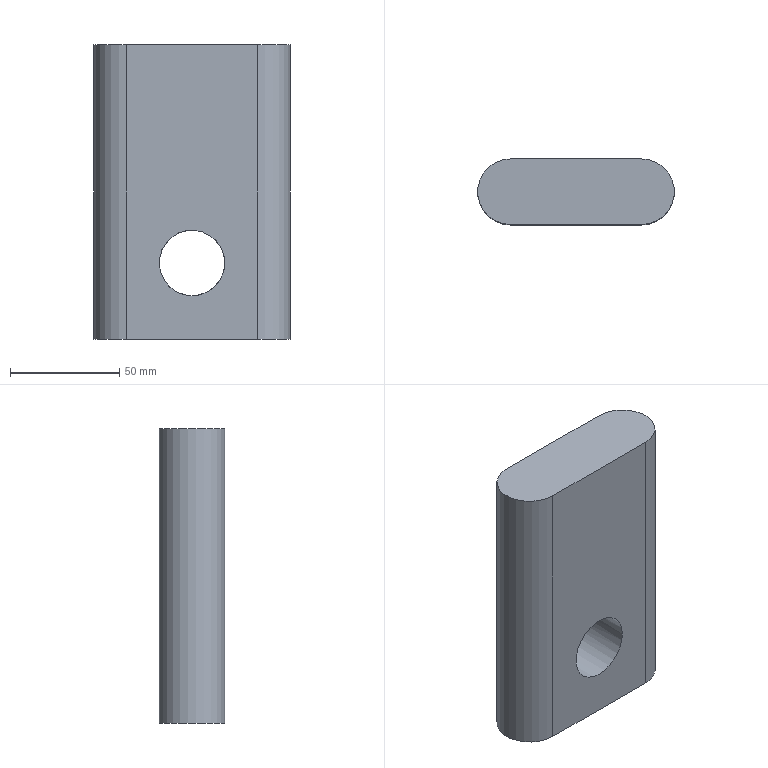Part | NX | features DATUM_CSYS 3, EXTRUDE 2, OFFSET_REGION 2, SKETCH 2, BLEND 1 | 1 solid | 7 faces | box 90 x 30 x 135 mm | volume 317220 mm3 | plane 4 | cylinder 3 | commonest cylinder face diameters 30 x3
STEP:
#1=CARTESIAN_POINT('',(15.,-15.,40.));
#2=VERTEX_POINT('',#1);
#3=CARTESIAN_POINT('',(0.,-15.,40.));
#4=DIRECTION('',(0.,-1.,0.));
#5=DIRECTION('',(1.,0.,0.));
#6=AXIS2_PLACEMENT_3D('',#3,#4,#5);
#7=CIRCLE('',#6,15.);
#8=EDGE_CURVE('',#2,#2,#7,.T.);
#9=ORIENTED_EDGE('',*,*,#8,.F.);
#10=EDGE_LOOP('',(#9));
#11=FACE_BOUND('',#10,.T.);
#12=CARTESIAN_POINT('',(-30.,-15.,5.));
#13=VERTEX_POINT('',#12);
#14=CARTESIAN_POINT('',(30.,-15.,5.));
#15=VERTEX_POINT('',#14);
#16=CARTESIAN_POINT('',(-45.,-15.,5.));
#17=DIRECTION('',(1.,0.,0.));
#18=VECTOR('',#17,1000.);
#19=LINE('',#16,#18);
#20=EDGE_CURVE('',#13,#15,#19,.T.);
#21=ORIENTED_EDGE('',*,*,#20,.T.);
#22=CARTESIAN_POINT('',(30.,-15.,140.));
#23=VERTEX_POINT('',#22);
#24=CARTESIAN_POINT('',(30.,-15.,100.));
#25=DIRECTION('',(0.,0.,-1.));
#26=VECTOR('',#25,1000.);
#27=LINE('',#24,#26);
#28=EDGE_CURVE('',#15,#23,#27,.F.);
#29=ORIENTED_EDGE('',*,*,#28,.T.);
#30=CARTESIAN_POINT('',(-30.,-15.,140.));
#31=VERTEX_POINT('',#30);
#32=CARTESIAN_POINT('',(-45.,-15.,140.));
#33=DIRECTION('',(1.,0.,0.));
#34=VECTOR('',#33,1000.);
#35=LINE('',#32,#34);
#36=EDGE_CURVE('',#31,#23,#35,.T.);
#37=ORIENTED_EDGE('',*,*,#36,.F.);
#38=CARTESIAN_POINT('',(-30.,-15.,100.));
#39=DIRECTION('',(0.,0.,-1.));
#40=VECTOR('',#39,1000.);
#41=LINE('',#38,#40);
#42=EDGE_CURVE('',#31,#13,#41,.T.);
#43=ORIENTED_EDGE('',*,*,#42,.T.);
#44=EDGE_LOOP('',(#21,#29,#37,#43));
#45=FACE_BOUND('',#44,.T.);
#46=CARTESIAN_POINT('',(-45.,-15.,100.));
#47=DIRECTION('',(0.,1.,0.));
#48=DIRECTION('',(0.,0.,1.));
#49=AXIS2_PLACEMENT_3D('',#46,#47,#48);
#50=PLANE('',#49);
#51=ADVANCED_FACE('',(#11,#45),#50,.F.);
#52=CARTESIAN_POINT('',(0.,15.,25.));
#53=VERTEX_POINT('',#52);
#54=CARTESIAN_POINT('',(0.,15.,40.));
#55=DIRECTION('',(0.,-1.,0.));
#56=DIRECTION('',(0.,0.,-1.));
#57=AXIS2_PLACEMENT_3D('',#54,#55,#56);
#58=CIRCLE('',#57,15.);
#59=EDGE_CURVE('',#53,#53,#58,.T.);
#60=ORIENTED_EDGE('',*,*,#59,.T.);
#61=EDGE_LOOP('',(#60));
#62=FACE_BOUND('',#61,.T.);
#63=CARTESIAN_POINT('',(30.,15.,140.));
#64=VERTEX_POINT('',#63);
#65=CARTESIAN_POINT('',(-30.,15.,140.));
#66=VERTEX_POINT('',#65);
#67=CARTESIAN_POINT('',(45.,15.,140.));
#68=DIRECTION('',(-1.,0.,0.));
#69=VECTOR('',#68,1000.);
#70=LINE('',#67,#69);
#71=EDGE_CURVE('',#64,#66,#70,.T.);
#72=ORIENTED_EDGE('',*,*,#71,.F.);
#73=CARTESIAN_POINT('',(30.,15.,5.));
#74=VERTEX_POINT('',#73);
#75=CARTESIAN_POINT('',(30.,15.,100.));
#76=DIRECTION('',(0.,0.,-1.));
#77=VECTOR('',#76,1000.);
#78=LINE('',#75,#77);
#79=EDGE_CURVE('',#64,#74,#78,.T.);
#80=ORIENTED_EDGE('',*,*,#79,.T.);
#81=CARTESIAN_POINT('',(-30.,15.,5.));
#82=VERTEX_POINT('',#81);
#83=CARTESIAN_POINT('',(45.,15.,5.));
#84=DIRECTION('',(-1.,0.,0.));
#85=VECTOR('',#84,1000.);
#86=LINE('',#83,#85);
#87=EDGE_CURVE('',#74,#82,#86,.T.);
#88=ORIENTED_EDGE('',*,*,#87,.T.);
#89=CARTESIAN_POINT('',(-30.,15.,100.));
#90=DIRECTION('',(0.,0.,-1.));
#91=VECTOR('',#90,1000.);
#92=LINE('',#89,#91);
#93=EDGE_CURVE('',#82,#66,#92,.F.);
#94=ORIENTED_EDGE('',*,*,#93,.T.);
#95=EDGE_LOOP('',(#72,#80,#88,#94));
#96=FACE_BOUND('',#95,.T.);
#97=CARTESIAN_POINT('',(45.,15.,100.));
#98=DIRECTION('',(0.,-1.,0.));
#99=DIRECTION('',(0.,0.,-1.));
#100=AXIS2_PLACEMENT_3D('',#97,#98,#99);
#101=PLANE('',#100);
#102=ADVANCED_FACE('',(#62,#96),#101,.F.);
#103=CARTESIAN_POINT('',(30.,0.,140.));
#104=DIRECTION('',(0.,0.,1.));
#105=DIRECTION('',(1.,0.,0.));
#106=AXIS2_PLACEMENT_3D('',#103,#104,#105);
#107=CIRCLE('',#106,15.);
#108=EDGE_CURVE('',#23,#64,#107,.T.);
#109=ORIENTED_EDGE('',*,*,#108,.T.);
#110=ORIENTED_EDGE('',*,*,#71,.T.);
#111=CARTESIAN_POINT('',(-30.,0.,140.));
#112=DIRECTION('',(0.,0.,1.));
#113=DIRECTION('',(1.,0.,0.));
#114=AXIS2_PLACEMENT_3D('',#111,#112,#113);
#115=CIRCLE('',#114,15.);
#116=EDGE_CURVE('',#66,#31,#115,.T.);
#117=ORIENTED_EDGE('',*,*,#116,.T.);
#118=ORIENTED_EDGE('',*,*,#36,.T.);
#119=EDGE_LOOP('',(#109,#110,#117,#118));
#120=FACE_BOUND('',#119,.T.);
#121=CARTESIAN_POINT('',(0.,0.,140.));
#122=DIRECTION('',(0.,0.,1.));
#123=DIRECTION('',(1.,0.,0.));
#124=AXIS2_PLACEMENT_3D('',#121,#122,#123);
#125=PLANE('',#124);
#126=ADVANCED_FACE('',(#120),#125,.T.);
#127=ORIENTED_EDGE('',*,*,#87,.F.);
#128=CARTESIAN_POINT('',(30.,0.,5.));
#129=DIRECTION('',(0.,0.,1.));
#130=DIRECTION('',(1.,0.,0.));
#131=AXIS2_PLACEMENT_3D('',#128,#129,#130);
#132=CIRCLE('',#131,15.);
#133=EDGE_CURVE('',#74,#15,#132,.F.);
#134=ORIENTED_EDGE('',*,*,#133,.T.);
#135=ORIENTED_EDGE('',*,*,#20,.F.);
#136=CARTESIAN_POINT('',(-30.,0.,5.));
#137=DIRECTION('',(0.,0.,1.));
#138=DIRECTION('',(1.,0.,0.));
#139=AXIS2_PLACEMENT_3D('',#136,#137,#138);
#140=CIRCLE('',#139,15.);
#141=EDGE_CURVE('',#13,#82,#140,.F.);
#142=ORIENTED_EDGE('',*,*,#141,.T.);
#143=EDGE_LOOP('',(#127,#134,#135,#142));
#144=FACE_BOUND('',#143,.T.);
#145=CARTESIAN_POINT('',(0.,0.,5.));
#146=DIRECTION('',(0.,0.,1.));
#147=DIRECTION('',(1.,0.,0.));
#148=AXIS2_PLACEMENT_3D('',#145,#146,#147);
#149=PLANE('',#148);
#150=ADVANCED_FACE('',(#144),#149,.F.);
#151=ORIENTED_EDGE('',*,*,#8,.T.);
#152=EDGE_LOOP('',(#151));
#153=FACE_BOUND('',#152,.T.);
#154=ORIENTED_EDGE('',*,*,#59,.F.);
#155=EDGE_LOOP('',(#154));
#156=FACE_BOUND('',#155,.T.);
#157=CARTESIAN_POINT('',(0.,85.,40.));
#158=DIRECTION('',(0.,-1.,0.));
#159=DIRECTION('',(0.,0.,-1.));
#160=AXIS2_PLACEMENT_3D('',#157,#158,#159);
#161=CYLINDRICAL_SURFACE('',#160,15.);
#162=ADVANCED_FACE('',(#153,#156),#161,.F.);
#163=ORIENTED_EDGE('',*,*,#133,.F.);
#164=ORIENTED_EDGE('',*,*,#79,.F.);
#165=ORIENTED_EDGE('',*,*,#108,.F.);
#166=ORIENTED_EDGE('',*,*,#28,.F.);
#167=EDGE_LOOP('',(#163,#164,#165,#166));
#168=FACE_BOUND('',#167,.T.);
#169=CARTESIAN_POINT('',(30.,0.,100.));
#170=DIRECTION('',(0.,0.,-1.));
#171=DIRECTION('',(-1.,0.,0.));
#172=AXIS2_PLACEMENT_3D('',#169,#170,#171);
#173=CYLINDRICAL_SURFACE('',#172,15.);
#174=ADVANCED_FACE('',(#168),#173,.T.);
#175=ORIENTED_EDGE('',*,*,#42,.F.);
#176=ORIENTED_EDGE('',*,*,#116,.F.);
#177=ORIENTED_EDGE('',*,*,#93,.F.);
#178=ORIENTED_EDGE('',*,*,#141,.F.);
#179=EDGE_LOOP('',(#175,#176,#177,#178));
#180=FACE_BOUND('',#179,.T.);
#181=CARTESIAN_POINT('',(-30.,0.,100.));
#182=DIRECTION('',(0.,0.,-1.));
#183=DIRECTION('',(-1.,0.,0.));
#184=AXIS2_PLACEMENT_3D('',#181,#182,#183);
#185=CYLINDRICAL_SURFACE('',#184,15.);
#186=ADVANCED_FACE('',(#180),#185,.T.);
#187=CLOSED_SHELL('',(#51,#102,#126,#150,#162,#174,#186));
#188=MANIFOLD_SOLID_BREP('',#187);
#189=(LENGTH_UNIT()NAMED_UNIT(*)SI_UNIT(.MILLI.,.METRE.));
#190=UNCERTAINTY_MEASURE_WITH_UNIT(LENGTH_MEASURE(0.00001),#189,'','');
#191=(NAMED_UNIT(*)PLANE_ANGLE_UNIT()SI_UNIT($,.RADIAN.));
#192=(NAMED_UNIT(*)SI_UNIT($,.STERADIAN.)SOLID_ANGLE_UNIT());
#193=(GEOMETRIC_REPRESENTATION_CONTEXT(3)GLOBAL_UNCERTAINTY_ASSIGNED_CONTEXT((#190))GLOBAL_UNIT_ASSIGNED_CONTEXT((#189,#191,#192))REPRESENTATION_CONTEXT('',''));
#194=ADVANCED_BREP_SHAPE_REPRESENTATION('',(#188),#193);